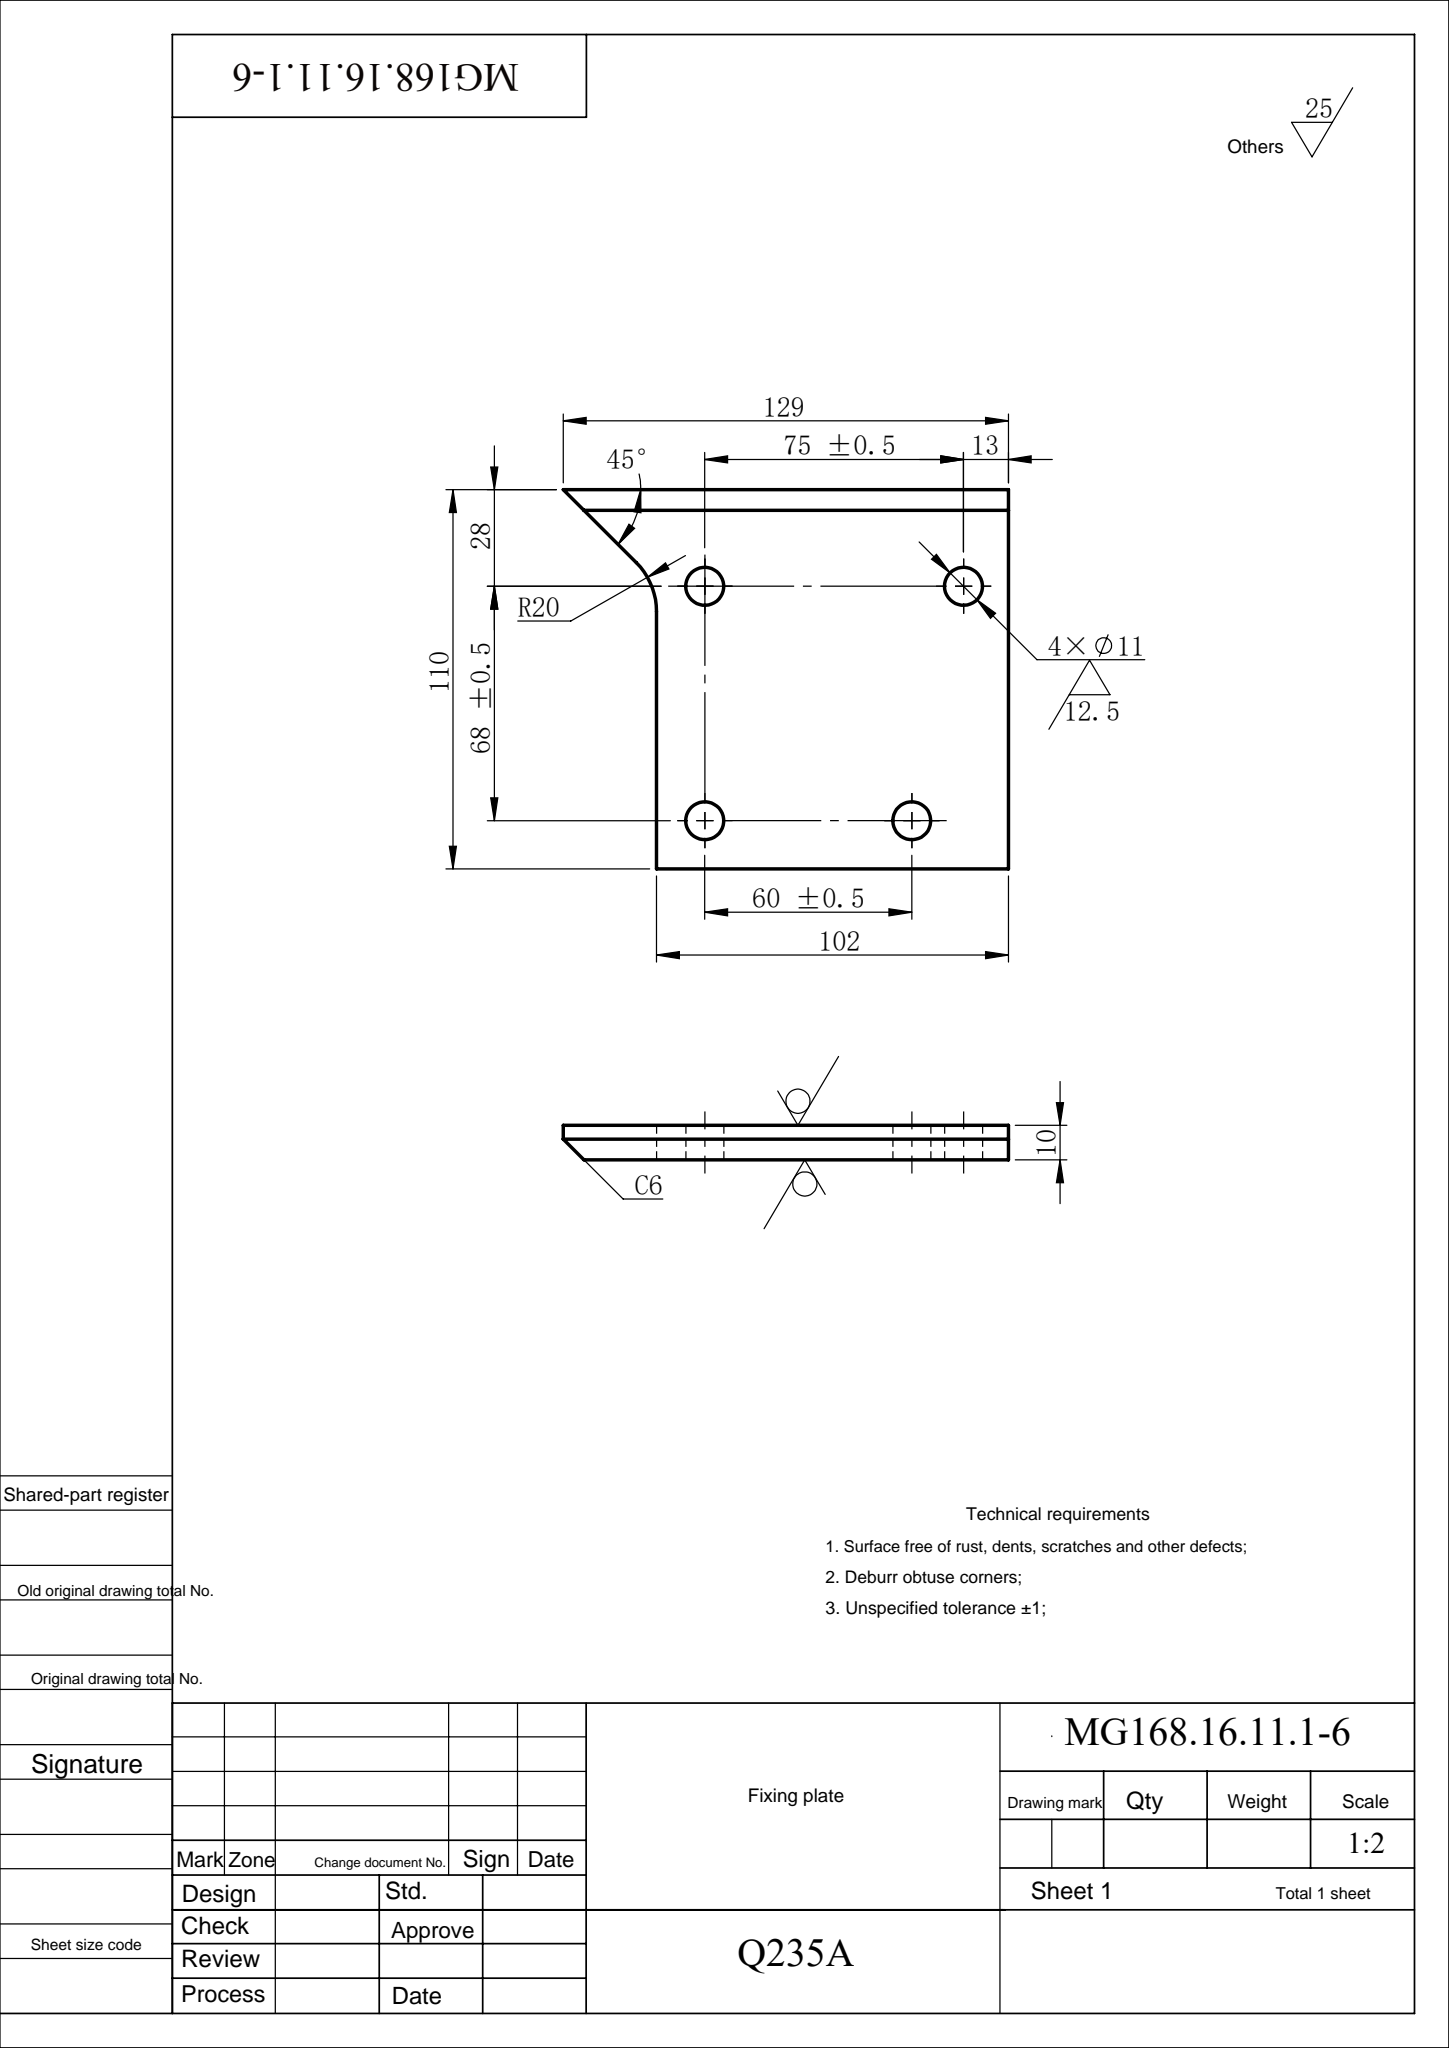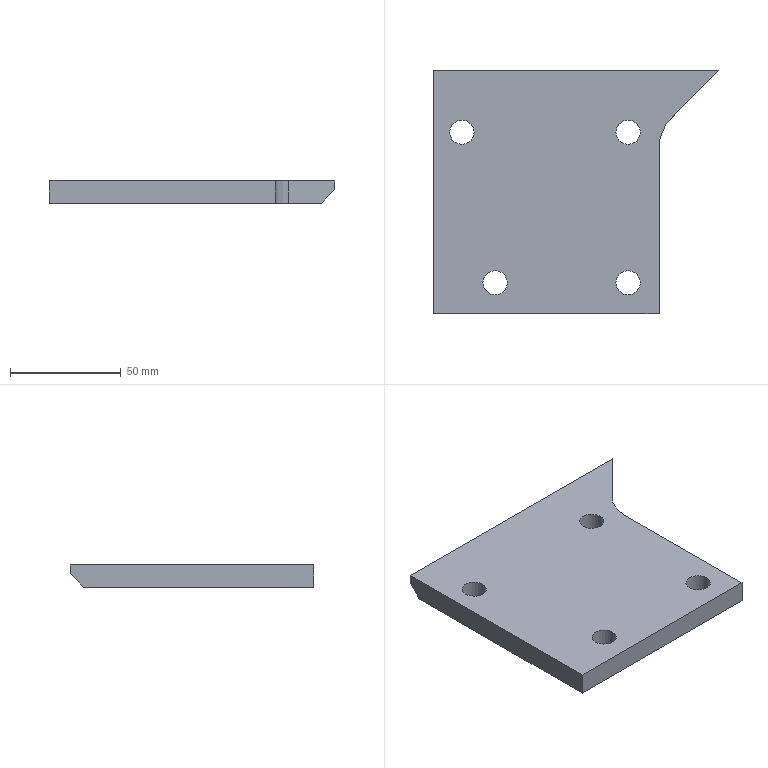Part | SolidWorks | features Chamfer 1, Extrusion 1, ICE 1 | 1 solid | 17 faces | box 129 x 110 x 10 mm | volume 109844 mm3 | cylinder 9 | plane 8 | commonest cylinder face diameters 11 x8 40 x1
STEP:
#1=CARTESIAN_POINT('',(24.5,68.,-5.));
#2=VERTEX_POINT('',#1);
#3=CARTESIAN_POINT('',(35.5,68.,-5.));
#4=VERTEX_POINT('',#3);
#5=CARTESIAN_POINT('',(30.,68.,-5.));
#6=DIRECTION('',(0.,0.,1.));
#7=DIRECTION('',(1.,0.,0.));
#8=AXIS2_PLACEMENT_3D('',#5,#6,#7);
#9=CIRCLE('',#8,5.5);
#10=EDGE_CURVE('',#2,#4,#9,.T.);
#11=ORIENTED_EDGE('',*,*,#10,.F.);
#12=CARTESIAN_POINT('',(24.5,68.,5.));
#13=VERTEX_POINT('',#12);
#14=CARTESIAN_POINT('',(24.5,68.,-5.));
#15=DIRECTION('',(0.,0.,1.));
#16=VECTOR('',#15,1000.);
#17=LINE('',#14,#16);
#18=EDGE_CURVE('',#2,#13,#17,.T.);
#19=ORIENTED_EDGE('',*,*,#18,.T.);
#20=CARTESIAN_POINT('',(35.5,68.,5.));
#21=VERTEX_POINT('',#20);
#22=CARTESIAN_POINT('',(30.,68.,5.));
#23=DIRECTION('',(0.,0.,1.));
#24=DIRECTION('',(1.,0.,0.));
#25=AXIS2_PLACEMENT_3D('',#22,#23,#24);
#26=CIRCLE('',#25,5.5);
#27=EDGE_CURVE('',#13,#21,#26,.T.);
#28=ORIENTED_EDGE('',*,*,#27,.T.);
#29=CARTESIAN_POINT('',(35.5,68.,-5.));
#30=DIRECTION('',(0.,0.,1.));
#31=VECTOR('',#30,1000.);
#32=LINE('',#29,#31);
#33=EDGE_CURVE('',#4,#21,#32,.T.);
#34=ORIENTED_EDGE('',*,*,#33,.F.);
#35=EDGE_LOOP('',(#11,#19,#28,#34));
#36=FACE_OUTER_BOUND('',#35,.T.);
#37=CARTESIAN_POINT('',(30.,68.,-5.));
#38=DIRECTION('',(0.,0.,1.));
#39=DIRECTION('',(1.,0.,0.));
#40=AXIS2_PLACEMENT_3D('',#37,#38,#39);
#41=CYLINDRICAL_SURFACE('',#40,5.5);
#42=ADVANCED_FACE('',(#36),#41,.F.);
#43=CARTESIAN_POINT('',(-50.5,68.,-5.));
#44=VERTEX_POINT('',#43);
#45=CARTESIAN_POINT('',(-39.5,68.,-5.));
#46=VERTEX_POINT('',#45);
#47=CARTESIAN_POINT('',(-45.,68.,-5.));
#48=DIRECTION('',(0.,0.,1.));
#49=DIRECTION('',(1.,0.,0.));
#50=AXIS2_PLACEMENT_3D('',#47,#48,#49);
#51=CIRCLE('',#50,5.5);
#52=EDGE_CURVE('',#44,#46,#51,.T.);
#53=ORIENTED_EDGE('',*,*,#52,.F.);
#54=CARTESIAN_POINT('',(-50.5,68.,5.));
#55=VERTEX_POINT('',#54);
#56=CARTESIAN_POINT('',(-50.5,68.,-5.));
#57=DIRECTION('',(0.,0.,1.));
#58=VECTOR('',#57,1000.);
#59=LINE('',#56,#58);
#60=EDGE_CURVE('',#44,#55,#59,.T.);
#61=ORIENTED_EDGE('',*,*,#60,.T.);
#62=CARTESIAN_POINT('',(-39.5,68.,5.));
#63=VERTEX_POINT('',#62);
#64=CARTESIAN_POINT('',(-45.,68.,5.));
#65=DIRECTION('',(0.,0.,1.));
#66=DIRECTION('',(1.,0.,0.));
#67=AXIS2_PLACEMENT_3D('',#64,#65,#66);
#68=CIRCLE('',#67,5.5);
#69=EDGE_CURVE('',#55,#63,#68,.T.);
#70=ORIENTED_EDGE('',*,*,#69,.T.);
#71=CARTESIAN_POINT('',(-39.5,68.,-5.));
#72=DIRECTION('',(0.,0.,1.));
#73=VECTOR('',#72,1000.);
#74=LINE('',#71,#73);
#75=EDGE_CURVE('',#46,#63,#74,.T.);
#76=ORIENTED_EDGE('',*,*,#75,.F.);
#77=EDGE_LOOP('',(#53,#61,#70,#76));
#78=FACE_OUTER_BOUND('',#77,.T.);
#79=CARTESIAN_POINT('',(-45.,68.,-5.));
#80=DIRECTION('',(0.,0.,1.));
#81=DIRECTION('',(1.,0.,0.));
#82=AXIS2_PLACEMENT_3D('',#79,#80,#81);
#83=CYLINDRICAL_SURFACE('',#82,5.5);
#84=ADVANCED_FACE('',(#78),#83,.F.);
#85=CARTESIAN_POINT('',(24.5,0.,-5.));
#86=VERTEX_POINT('',#85);
#87=CARTESIAN_POINT('',(35.5,0.,-5.));
#88=VERTEX_POINT('',#87);
#89=CARTESIAN_POINT('',(30.,0.,-5.));
#90=DIRECTION('',(0.,0.,1.));
#91=DIRECTION('',(1.,0.,0.));
#92=AXIS2_PLACEMENT_3D('',#89,#90,#91);
#93=CIRCLE('',#92,5.5);
#94=EDGE_CURVE('',#86,#88,#93,.T.);
#95=ORIENTED_EDGE('',*,*,#94,.F.);
#96=CARTESIAN_POINT('',(24.5,0.,5.));
#97=VERTEX_POINT('',#96);
#98=CARTESIAN_POINT('',(24.5,0.,-5.));
#99=DIRECTION('',(0.,0.,1.));
#100=VECTOR('',#99,1000.);
#101=LINE('',#98,#100);
#102=EDGE_CURVE('',#86,#97,#101,.T.);
#103=ORIENTED_EDGE('',*,*,#102,.T.);
#104=CARTESIAN_POINT('',(35.5,0.,5.));
#105=VERTEX_POINT('',#104);
#106=CARTESIAN_POINT('',(30.,0.,5.));
#107=DIRECTION('',(0.,0.,1.));
#108=DIRECTION('',(1.,0.,0.));
#109=AXIS2_PLACEMENT_3D('',#106,#107,#108);
#110=CIRCLE('',#109,5.5);
#111=EDGE_CURVE('',#97,#105,#110,.T.);
#112=ORIENTED_EDGE('',*,*,#111,.T.);
#113=CARTESIAN_POINT('',(35.5,0.,-5.));
#114=DIRECTION('',(0.,0.,1.));
#115=VECTOR('',#114,1000.);
#116=LINE('',#113,#115);
#117=EDGE_CURVE('',#88,#105,#116,.T.);
#118=ORIENTED_EDGE('',*,*,#117,.F.);
#119=EDGE_LOOP('',(#95,#103,#112,#118));
#120=FACE_OUTER_BOUND('',#119,.T.);
#121=CARTESIAN_POINT('',(30.,0.,-5.));
#122=DIRECTION('',(0.,0.,1.));
#123=DIRECTION('',(1.,0.,0.));
#124=AXIS2_PLACEMENT_3D('',#121,#122,#123);
#125=CYLINDRICAL_SURFACE('',#124,5.5);
#126=ADVANCED_FACE('',(#120),#125,.F.);
#127=CARTESIAN_POINT('',(-35.5,0.,-5.));
#128=VERTEX_POINT('',#127);
#129=CARTESIAN_POINT('',(-24.5,0.,-5.));
#130=VERTEX_POINT('',#129);
#131=CARTESIAN_POINT('',(-30.,0.,-5.));
#132=DIRECTION('',(0.,0.,1.));
#133=DIRECTION('',(1.,0.,0.));
#134=AXIS2_PLACEMENT_3D('',#131,#132,#133);
#135=CIRCLE('',#134,5.5);
#136=EDGE_CURVE('',#128,#130,#135,.T.);
#137=ORIENTED_EDGE('',*,*,#136,.F.);
#138=CARTESIAN_POINT('',(-35.5,0.,5.));
#139=VERTEX_POINT('',#138);
#140=CARTESIAN_POINT('',(-35.5,0.,-5.));
#141=DIRECTION('',(0.,0.,1.));
#142=VECTOR('',#141,1000.);
#143=LINE('',#140,#142);
#144=EDGE_CURVE('',#128,#139,#143,.T.);
#145=ORIENTED_EDGE('',*,*,#144,.T.);
#146=CARTESIAN_POINT('',(-24.5,0.,5.));
#147=VERTEX_POINT('',#146);
#148=CARTESIAN_POINT('',(-30.,0.,5.));
#149=DIRECTION('',(0.,0.,1.));
#150=DIRECTION('',(1.,0.,0.));
#151=AXIS2_PLACEMENT_3D('',#148,#149,#150);
#152=CIRCLE('',#151,5.5);
#153=EDGE_CURVE('',#139,#147,#152,.T.);
#154=ORIENTED_EDGE('',*,*,#153,.T.);
#155=CARTESIAN_POINT('',(-24.5,0.,-5.));
#156=DIRECTION('',(0.,0.,1.));
#157=VECTOR('',#156,1000.);
#158=LINE('',#155,#157);
#159=EDGE_CURVE('',#130,#147,#158,.T.);
#160=ORIENTED_EDGE('',*,*,#159,.F.);
#161=EDGE_LOOP('',(#137,#145,#154,#160));
#162=FACE_OUTER_BOUND('',#161,.T.);
#163=CARTESIAN_POINT('',(-30.,0.,-5.));
#164=DIRECTION('',(0.,0.,1.));
#165=DIRECTION('',(1.,0.,0.));
#166=AXIS2_PLACEMENT_3D('',#163,#164,#165);
#167=CYLINDRICAL_SURFACE('',#166,5.5);
#168=ADVANCED_FACE('',(#162),#167,.F.);
#169=CARTESIAN_POINT('',(-58.,96.,5.));
#170=VERTEX_POINT('',#169);
#171=CARTESIAN_POINT('',(-58.,96.,1.));
#172=VERTEX_POINT('',#171);
#173=CARTESIAN_POINT('',(-58.,96.,5.));
#174=DIRECTION('',(0.,0.,-1.));
#175=VECTOR('',#174,1000.);
#176=LINE('',#173,#175);
#177=EDGE_CURVE('',#170,#172,#176,.T.);
#178=ORIENTED_EDGE('',*,*,#177,.T.);
#179=CARTESIAN_POINT('',(-58.,90.,-5.));
#180=VERTEX_POINT('',#179);
#181=CARTESIAN_POINT('',(-58.,96.,1.));
#182=DIRECTION('',(0.,-0.7071,-0.7071));
#183=VECTOR('',#182,1000.);
#184=LINE('',#181,#183);
#185=EDGE_CURVE('',#172,#180,#184,.T.);
#186=ORIENTED_EDGE('',*,*,#185,.T.);
#187=CARTESIAN_POINT('',(-58.,-14.,-5.));
#188=VERTEX_POINT('',#187);
#189=CARTESIAN_POINT('',(-58.,96.,-5.));
#190=DIRECTION('',(0.,-1.,0.));
#191=VECTOR('',#190,1000.);
#192=LINE('',#189,#191);
#193=EDGE_CURVE('',#180,#188,#192,.T.);
#194=ORIENTED_EDGE('',*,*,#193,.T.);
#195=CARTESIAN_POINT('',(-58.,-14.,5.));
#196=VERTEX_POINT('',#195);
#197=CARTESIAN_POINT('',(-58.,-14.,5.));
#198=DIRECTION('',(0.,0.,-1.));
#199=VECTOR('',#198,1000.);
#200=LINE('',#197,#199);
#201=EDGE_CURVE('',#196,#188,#200,.T.);
#202=ORIENTED_EDGE('',*,*,#201,.F.);
#203=CARTESIAN_POINT('',(-58.,96.,5.));
#204=DIRECTION('',(0.,-1.,0.));
#205=VECTOR('',#204,1000.);
#206=LINE('',#203,#205);
#207=EDGE_CURVE('',#170,#196,#206,.T.);
#208=ORIENTED_EDGE('',*,*,#207,.F.);
#209=EDGE_LOOP('',(#178,#186,#194,#202,#208));
#210=FACE_OUTER_BOUND('',#209,.T.);
#211=CARTESIAN_POINT('',(-58.,96.,5.));
#212=DIRECTION('',(1.,0.,0.));
#213=DIRECTION('',(0.,1.,0.));
#214=AXIS2_PLACEMENT_3D('',#211,#212,#213);
#215=PLANE('',#214);
#216=ADVANCED_FACE('',(#210),#215,.F.);
#217=CARTESIAN_POINT('',(44.,-14.,-5.));
#218=VERTEX_POINT('',#217);
#219=CARTESIAN_POINT('',(-58.,-14.,-5.));
#220=DIRECTION('',(1.,0.,0.));
#221=VECTOR('',#220,1000.);
#222=LINE('',#219,#221);
#223=EDGE_CURVE('',#188,#218,#222,.T.);
#224=ORIENTED_EDGE('',*,*,#223,.T.);
#225=CARTESIAN_POINT('',(44.,-14.,5.));
#226=VERTEX_POINT('',#225);
#227=CARTESIAN_POINT('',(44.,-14.,5.));
#228=DIRECTION('',(0.,0.,-1.));
#229=VECTOR('',#228,1000.);
#230=LINE('',#227,#229);
#231=EDGE_CURVE('',#226,#218,#230,.T.);
#232=ORIENTED_EDGE('',*,*,#231,.F.);
#233=CARTESIAN_POINT('',(-58.,-14.,5.));
#234=DIRECTION('',(1.,0.,0.));
#235=VECTOR('',#234,1000.);
#236=LINE('',#233,#235);
#237=EDGE_CURVE('',#196,#226,#236,.T.);
#238=ORIENTED_EDGE('',*,*,#237,.F.);
#239=ORIENTED_EDGE('',*,*,#201,.T.);
#240=EDGE_LOOP('',(#224,#232,#238,#239));
#241=FACE_OUTER_BOUND('',#240,.T.);
#242=CARTESIAN_POINT('',(-58.,-14.,5.));
#243=DIRECTION('',(0.,1.,0.));
#244=DIRECTION('',(-1.,0.,0.));
#245=AXIS2_PLACEMENT_3D('',#242,#243,#244);
#246=PLANE('',#245);
#247=ADVANCED_FACE('',(#241),#246,.F.);
#248=CARTESIAN_POINT('',(44.,60.716,-5.));
#249=VERTEX_POINT('',#248);
#250=CARTESIAN_POINT('',(44.,60.716,-5.));
#251=DIRECTION('',(0.,1.,0.));
#252=VECTOR('',#251,1000.);
#253=LINE('',#250,#252);
#254=EDGE_CURVE('',#218,#249,#253,.T.);
#255=ORIENTED_EDGE('',*,*,#254,.T.);
#256=CARTESIAN_POINT('',(44.,60.716,5.));
#257=VERTEX_POINT('',#256);
#258=CARTESIAN_POINT('',(44.,60.716,5.));
#259=DIRECTION('',(0.,0.,-1.));
#260=VECTOR('',#259,1000.);
#261=LINE('',#258,#260);
#262=EDGE_CURVE('',#257,#249,#261,.T.);
#263=ORIENTED_EDGE('',*,*,#262,.F.);
#264=CARTESIAN_POINT('',(44.,60.716,5.));
#265=DIRECTION('',(0.,1.,0.));
#266=VECTOR('',#265,1000.);
#267=LINE('',#264,#266);
#268=EDGE_CURVE('',#226,#257,#267,.T.);
#269=ORIENTED_EDGE('',*,*,#268,.F.);
#270=ORIENTED_EDGE('',*,*,#231,.T.);
#271=EDGE_LOOP('',(#255,#263,#269,#270));
#272=FACE_OUTER_BOUND('',#271,.T.);
#273=CARTESIAN_POINT('',(44.,60.716,5.));
#274=DIRECTION('',(-1.,0.,0.));
#275=DIRECTION('',(0.,0.,1.));
#276=AXIS2_PLACEMENT_3D('',#273,#274,#275);
#277=PLANE('',#276);
#278=ADVANCED_FACE('',(#272),#277,.F.);
#279=CARTESIAN_POINT('',(49.858,74.858,-5.));
#280=VERTEX_POINT('',#279);
#281=CARTESIAN_POINT('',(64.,60.716,-5.));
#282=DIRECTION('',(0.,0.,-1.));
#283=DIRECTION('',(-1.,0.,0.));
#284=AXIS2_PLACEMENT_3D('',#281,#282,#283);
#285=CIRCLE('',#284,20.);
#286=EDGE_CURVE('',#249,#280,#285,.T.);
#287=ORIENTED_EDGE('',*,*,#286,.T.);
#288=CARTESIAN_POINT('',(49.858,74.858,5.));
#289=VERTEX_POINT('',#288);
#290=CARTESIAN_POINT('',(49.858,74.858,5.));
#291=DIRECTION('',(0.,0.,-1.));
#292=VECTOR('',#291,1000.);
#293=LINE('',#290,#292);
#294=EDGE_CURVE('',#289,#280,#293,.T.);
#295=ORIENTED_EDGE('',*,*,#294,.F.);
#296=CARTESIAN_POINT('',(64.,60.716,5.));
#297=DIRECTION('',(0.,0.,-1.));
#298=DIRECTION('',(-1.,0.,0.));
#299=AXIS2_PLACEMENT_3D('',#296,#297,#298);
#300=CIRCLE('',#299,20.);
#301=EDGE_CURVE('',#257,#289,#300,.T.);
#302=ORIENTED_EDGE('',*,*,#301,.F.);
#303=ORIENTED_EDGE('',*,*,#262,.T.);
#304=EDGE_LOOP('',(#287,#295,#302,#303));
#305=FACE_OUTER_BOUND('',#304,.T.);
#306=CARTESIAN_POINT('',(64.,60.716,5.));
#307=DIRECTION('',(0.,0.,-1.));
#308=DIRECTION('',(-1.,0.,0.));
#309=AXIS2_PLACEMENT_3D('',#306,#307,#308);
#310=CYLINDRICAL_SURFACE('',#309,20.);
#311=ADVANCED_FACE('',(#305),#310,.F.);
#312=CARTESIAN_POINT('',(65.,90.,-5.));
#313=VERTEX_POINT('',#312);
#314=CARTESIAN_POINT('',(71.,96.,-5.));
#315=DIRECTION('',(0.7071,0.7071,0.));
#316=VECTOR('',#315,1000.);
#317=LINE('',#314,#316);
#318=EDGE_CURVE('',#280,#313,#317,.T.);
#319=ORIENTED_EDGE('',*,*,#318,.T.);
#320=CARTESIAN_POINT('',(71.,96.,1.));
#321=VERTEX_POINT('',#320);
#322=CARTESIAN_POINT('',(28.,53.,-42.));
#323=DIRECTION('',(0.5774,0.5774,0.5774));
#324=VECTOR('',#323,1000.);
#325=LINE('',#322,#324);
#326=EDGE_CURVE('',#313,#321,#325,.T.);
#327=ORIENTED_EDGE('',*,*,#326,.T.);
#328=CARTESIAN_POINT('',(71.,96.,5.));
#329=VERTEX_POINT('',#328);
#330=CARTESIAN_POINT('',(71.,96.,5.));
#331=DIRECTION('',(0.,0.,-1.));
#332=VECTOR('',#331,1000.);
#333=LINE('',#330,#332);
#334=EDGE_CURVE('',#329,#321,#333,.T.);
#335=ORIENTED_EDGE('',*,*,#334,.F.);
#336=CARTESIAN_POINT('',(71.,96.,5.));
#337=DIRECTION('',(0.7071,0.7071,0.));
#338=VECTOR('',#337,1000.);
#339=LINE('',#336,#338);
#340=EDGE_CURVE('',#289,#329,#339,.T.);
#341=ORIENTED_EDGE('',*,*,#340,.F.);
#342=ORIENTED_EDGE('',*,*,#294,.T.);
#343=EDGE_LOOP('',(#319,#327,#335,#341,#342));
#344=FACE_OUTER_BOUND('',#343,.T.);
#345=CARTESIAN_POINT('',(71.,96.,5.));
#346=DIRECTION('',(-0.7071,0.7071,0.));
#347=DIRECTION('',(-0.7071,-0.7071,0.));
#348=AXIS2_PLACEMENT_3D('',#345,#346,#347);
#349=PLANE('',#348);
#350=ADVANCED_FACE('',(#344),#349,.F.);
#351=ORIENTED_EDGE('',*,*,#334,.T.);
#352=CARTESIAN_POINT('',(-58.,96.,1.));
#353=DIRECTION('',(-1.,0.,0.));
#354=VECTOR('',#353,1000.);
#355=LINE('',#352,#354);
#356=EDGE_CURVE('',#321,#172,#355,.T.);
#357=ORIENTED_EDGE('',*,*,#356,.T.);
#358=ORIENTED_EDGE('',*,*,#177,.F.);
#359=CARTESIAN_POINT('',(-58.,96.,5.));
#360=DIRECTION('',(-1.,0.,0.));
#361=VECTOR('',#360,1000.);
#362=LINE('',#359,#361);
#363=EDGE_CURVE('',#329,#170,#362,.T.);
#364=ORIENTED_EDGE('',*,*,#363,.F.);
#365=EDGE_LOOP('',(#351,#357,#358,#364));
#366=FACE_OUTER_BOUND('',#365,.T.);
#367=CARTESIAN_POINT('',(-58.,96.,5.));
#368=DIRECTION('',(0.,-1.,0.));
#369=DIRECTION('',(0.,0.,-1.));
#370=AXIS2_PLACEMENT_3D('',#367,#368,#369);
#371=PLANE('',#370);
#372=ADVANCED_FACE('',(#366),#371,.F.);
#373=CARTESIAN_POINT('',(30.,68.,5.));
#374=DIRECTION('',(0.,0.,1.));
#375=DIRECTION('',(1.,0.,0.));
#376=AXIS2_PLACEMENT_3D('',#373,#374,#375);
#377=CIRCLE('',#376,5.5);
#378=EDGE_CURVE('',#21,#13,#377,.T.);
#379=ORIENTED_EDGE('',*,*,#378,.F.);
#380=ORIENTED_EDGE('',*,*,#27,.F.);
#381=EDGE_LOOP('',(#379,#380));
#382=FACE_BOUND('',#381,.T.);
#383=CARTESIAN_POINT('',(-45.,68.,5.));
#384=DIRECTION('',(0.,0.,1.));
#385=DIRECTION('',(1.,0.,0.));
#386=AXIS2_PLACEMENT_3D('',#383,#384,#385);
#387=CIRCLE('',#386,5.5);
#388=EDGE_CURVE('',#63,#55,#387,.T.);
#389=ORIENTED_EDGE('',*,*,#388,.F.);
#390=ORIENTED_EDGE('',*,*,#69,.F.);
#391=EDGE_LOOP('',(#389,#390));
#392=FACE_BOUND('',#391,.T.);
#393=CARTESIAN_POINT('',(30.,0.,5.));
#394=DIRECTION('',(0.,0.,1.));
#395=DIRECTION('',(1.,0.,0.));
#396=AXIS2_PLACEMENT_3D('',#393,#394,#395);
#397=CIRCLE('',#396,5.5);
#398=EDGE_CURVE('',#105,#97,#397,.T.);
#399=ORIENTED_EDGE('',*,*,#398,.F.);
#400=ORIENTED_EDGE('',*,*,#111,.F.);
#401=EDGE_LOOP('',(#399,#400));
#402=FACE_BOUND('',#401,.T.);
#403=CARTESIAN_POINT('',(-30.,0.,5.));
#404=DIRECTION('',(0.,0.,1.));
#405=DIRECTION('',(1.,0.,0.));
#406=AXIS2_PLACEMENT_3D('',#403,#404,#405);
#407=CIRCLE('',#406,5.5);
#408=EDGE_CURVE('',#147,#139,#407,.T.);
#409=ORIENTED_EDGE('',*,*,#408,.F.);
#410=ORIENTED_EDGE('',*,*,#153,.F.);
#411=EDGE_LOOP('',(#409,#410));
#412=FACE_BOUND('',#411,.T.);
#413=ORIENTED_EDGE('',*,*,#207,.T.);
#414=ORIENTED_EDGE('',*,*,#237,.T.);
#415=ORIENTED_EDGE('',*,*,#268,.T.);
#416=ORIENTED_EDGE('',*,*,#301,.T.);
#417=ORIENTED_EDGE('',*,*,#340,.T.);
#418=ORIENTED_EDGE('',*,*,#363,.T.);
#419=EDGE_LOOP('',(#413,#414,#415,#416,#417,#418));
#420=FACE_OUTER_BOUND('',#419,.T.);
#421=CARTESIAN_POINT('',(64.,60.716,5.));
#422=DIRECTION('',(0.,0.,-1.));
#423=DIRECTION('',(-1.,0.,0.));
#424=AXIS2_PLACEMENT_3D('',#421,#422,#423);
#425=PLANE('',#424);
#426=ADVANCED_FACE('',(#382,#392,#402,#412,#420),#425,.F.);
#427=CARTESIAN_POINT('',(30.,68.,-5.));
#428=DIRECTION('',(0.,0.,1.));
#429=DIRECTION('',(1.,0.,0.));
#430=AXIS2_PLACEMENT_3D('',#427,#428,#429);
#431=CIRCLE('',#430,5.5);
#432=EDGE_CURVE('',#4,#2,#431,.T.);
#433=ORIENTED_EDGE('',*,*,#432,.T.);
#434=ORIENTED_EDGE('',*,*,#10,.T.);
#435=EDGE_LOOP('',(#433,#434));
#436=FACE_BOUND('',#435,.T.);
#437=CARTESIAN_POINT('',(-45.,68.,-5.));
#438=DIRECTION('',(0.,0.,1.));
#439=DIRECTION('',(1.,0.,0.));
#440=AXIS2_PLACEMENT_3D('',#437,#438,#439);
#441=CIRCLE('',#440,5.5);
#442=EDGE_CURVE('',#46,#44,#441,.T.);
#443=ORIENTED_EDGE('',*,*,#442,.T.);
#444=ORIENTED_EDGE('',*,*,#52,.T.);
#445=EDGE_LOOP('',(#443,#444));
#446=FACE_BOUND('',#445,.T.);
#447=CARTESIAN_POINT('',(30.,0.,-5.));
#448=DIRECTION('',(0.,0.,1.));
#449=DIRECTION('',(1.,0.,0.));
#450=AXIS2_PLACEMENT_3D('',#447,#448,#449);
#451=CIRCLE('',#450,5.5);
#452=EDGE_CURVE('',#88,#86,#451,.T.);
#453=ORIENTED_EDGE('',*,*,#452,.T.);
#454=ORIENTED_EDGE('',*,*,#94,.T.);
#455=EDGE_LOOP('',(#453,#454));
#456=FACE_BOUND('',#455,.T.);
#457=CARTESIAN_POINT('',(-30.,0.,-5.));
#458=DIRECTION('',(0.,0.,1.));
#459=DIRECTION('',(1.,0.,0.));
#460=AXIS2_PLACEMENT_3D('',#457,#458,#459);
#461=CIRCLE('',#460,5.5);
#462=EDGE_CURVE('',#130,#128,#461,.T.);
#463=ORIENTED_EDGE('',*,*,#462,.T.);
#464=ORIENTED_EDGE('',*,*,#136,.T.);
#465=EDGE_LOOP('',(#463,#464));
#466=FACE_BOUND('',#465,.T.);
#467=ORIENTED_EDGE('',*,*,#193,.F.);
#468=CARTESIAN_POINT('',(71.,90.,-5.));
#469=DIRECTION('',(1.,0.,0.));
#470=VECTOR('',#469,1000.);
#471=LINE('',#468,#470);
#472=EDGE_CURVE('',#180,#313,#471,.T.);
#473=ORIENTED_EDGE('',*,*,#472,.T.);
#474=ORIENTED_EDGE('',*,*,#318,.F.);
#475=ORIENTED_EDGE('',*,*,#286,.F.);
#476=ORIENTED_EDGE('',*,*,#254,.F.);
#477=ORIENTED_EDGE('',*,*,#223,.F.);
#478=EDGE_LOOP('',(#467,#473,#474,#475,#476,#477));
#479=FACE_OUTER_BOUND('',#478,.T.);
#480=CARTESIAN_POINT('',(64.,60.716,-5.));
#481=DIRECTION('',(0.,0.,-1.));
#482=DIRECTION('',(-1.,0.,0.));
#483=AXIS2_PLACEMENT_3D('',#480,#481,#482);
#484=PLANE('',#483);
#485=ADVANCED_FACE('',(#436,#446,#456,#466,#479),#484,.T.);
#486=ORIENTED_EDGE('',*,*,#144,.F.);
#487=ORIENTED_EDGE('',*,*,#462,.F.);
#488=ORIENTED_EDGE('',*,*,#159,.T.);
#489=ORIENTED_EDGE('',*,*,#408,.T.);
#490=EDGE_LOOP('',(#486,#487,#488,#489));
#491=FACE_OUTER_BOUND('',#490,.T.);
#492=CARTESIAN_POINT('',(-30.,0.,-5.));
#493=DIRECTION('',(0.,0.,1.));
#494=DIRECTION('',(1.,0.,0.));
#495=AXIS2_PLACEMENT_3D('',#492,#493,#494);
#496=CYLINDRICAL_SURFACE('',#495,5.5);
#497=ADVANCED_FACE('',(#491),#496,.F.);
#498=ORIENTED_EDGE('',*,*,#102,.F.);
#499=ORIENTED_EDGE('',*,*,#452,.F.);
#500=ORIENTED_EDGE('',*,*,#117,.T.);
#501=ORIENTED_EDGE('',*,*,#398,.T.);
#502=EDGE_LOOP('',(#498,#499,#500,#501));
#503=FACE_OUTER_BOUND('',#502,.T.);
#504=CARTESIAN_POINT('',(30.,0.,-5.));
#505=DIRECTION('',(0.,0.,1.));
#506=DIRECTION('',(1.,0.,0.));
#507=AXIS2_PLACEMENT_3D('',#504,#505,#506);
#508=CYLINDRICAL_SURFACE('',#507,5.5);
#509=ADVANCED_FACE('',(#503),#508,.F.);
#510=ORIENTED_EDGE('',*,*,#60,.F.);
#511=ORIENTED_EDGE('',*,*,#442,.F.);
#512=ORIENTED_EDGE('',*,*,#75,.T.);
#513=ORIENTED_EDGE('',*,*,#388,.T.);
#514=EDGE_LOOP('',(#510,#511,#512,#513));
#515=FACE_OUTER_BOUND('',#514,.T.);
#516=CARTESIAN_POINT('',(-45.,68.,-5.));
#517=DIRECTION('',(0.,0.,1.));
#518=DIRECTION('',(1.,0.,0.));
#519=AXIS2_PLACEMENT_3D('',#516,#517,#518);
#520=CYLINDRICAL_SURFACE('',#519,5.5);
#521=ADVANCED_FACE('',(#515),#520,.F.);
#522=ORIENTED_EDGE('',*,*,#18,.F.);
#523=ORIENTED_EDGE('',*,*,#432,.F.);
#524=ORIENTED_EDGE('',*,*,#33,.T.);
#525=ORIENTED_EDGE('',*,*,#378,.T.);
#526=EDGE_LOOP('',(#522,#523,#524,#525));
#527=FACE_OUTER_BOUND('',#526,.T.);
#528=CARTESIAN_POINT('',(30.,68.,-5.));
#529=DIRECTION('',(0.,0.,1.));
#530=DIRECTION('',(1.,0.,0.));
#531=AXIS2_PLACEMENT_3D('',#528,#529,#530);
#532=CYLINDRICAL_SURFACE('',#531,5.5);
#533=ADVANCED_FACE('',(#527),#532,.F.);
#534=ORIENTED_EDGE('',*,*,#326,.F.);
#535=ORIENTED_EDGE('',*,*,#472,.F.);
#536=ORIENTED_EDGE('',*,*,#185,.F.);
#537=ORIENTED_EDGE('',*,*,#356,.F.);
#538=EDGE_LOOP('',(#534,#535,#536,#537));
#539=FACE_OUTER_BOUND('',#538,.T.);
#540=CARTESIAN_POINT('',(-58.,96.,1.));
#541=DIRECTION('',(0.,0.7071,-0.7071));
#542=DIRECTION('',(1.,0.,0.));
#543=AXIS2_PLACEMENT_3D('',#540,#541,#542);
#544=PLANE('',#543);
#545=ADVANCED_FACE('',(#539),#544,.T.);
#546=CLOSED_SHELL('',(#42,#84,#126,#168,#216,#247,#278,#311,#350,#372,#426,#485,#497,#509,#521,#533,#545));
#547=MANIFOLD_SOLID_BREP('',#546);
#548=CARTESIAN_POINT('',(0.,0.,0.));
#549=DIRECTION('',(0.,0.,1.));
#550=DIRECTION('',(1.,0.,0.));
#551=AXIS2_PLACEMENT_3D('',#548,#549,#550);
#552=(LENGTH_UNIT()NAMED_UNIT(*)SI_UNIT(.MILLI.,.METRE.));
#553=UNCERTAINTY_MEASURE_WITH_UNIT(LENGTH_MEASURE(0.00001),#552,'','');
#554=(NAMED_UNIT(*)PLANE_ANGLE_UNIT()SI_UNIT($,.RADIAN.));
#555=(NAMED_UNIT(*)SI_UNIT($,.STERADIAN.)SOLID_ANGLE_UNIT());
#556=(GEOMETRIC_REPRESENTATION_CONTEXT(3)GLOBAL_UNCERTAINTY_ASSIGNED_CONTEXT((#553))GLOBAL_UNIT_ASSIGNED_CONTEXT((#552,#554,#555))REPRESENTATION_CONTEXT('',''));
#557=ADVANCED_BREP_SHAPE_REPRESENTATION('',(#547,#551),#556);